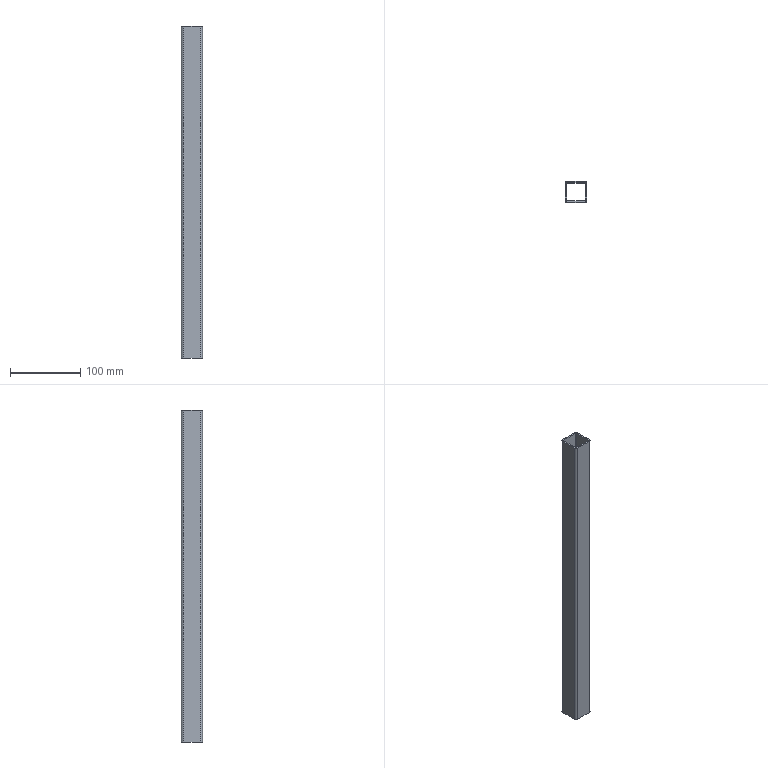Part | STEP file | DIN EN 10305-5 - 30 x 30 x 2  - 473 | 1 solid | 18 faces | box 30 x 30 x 473 mm | volume 102704 mm3 | plane 10 | cylinder 8 | commonest cylinder face diameters 2 x4 6 x4
STEP:
#1=CARTESIAN_POINT('',(0.,0.,0.));
#2=DIRECTION('',(0.,0.,1.));
#3=DIRECTION('',(1.,0.,0.));
#4=AXIS2_PLACEMENT_3D('',#1,#2,#3);
#5=CARTESIAN_POINT('',(-12.,-13.,473.));
#6=VERTEX_POINT('',#5);
#7=CARTESIAN_POINT('',(12.,-13.,473.));
#8=VERTEX_POINT('',#7);
#9=CARTESIAN_POINT('',(6.,-13.,473.));
#10=DIRECTION('',(1.,0.,0.));
#11=VECTOR('',#10,1.);
#12=LINE('',#9,#11);
#13=CARTESIAN_POINT('',(12.,-13.,0.));
#14=DIRECTION('',(0.,-1.,0.));
#15=DIRECTION('',(0.,0.,-1.));
#16=AXIS2_PLACEMENT_3D('',#13,#14,#15);
#17=PLANE('',#16);
#18=CARTESIAN_POINT('',(-473.,-6.));
#19=DIRECTION('',(0.,1.));
#20=VECTOR('',#19,1.);
#21=LINE('',#18,#20);
#22=(GEOMETRIC_REPRESENTATION_CONTEXT(2)PARAMETRIC_REPRESENTATION_CONTEXT()REPRESENTATION_CONTEXT('',''));
#23=DEFINITIONAL_REPRESENTATION('',(#21),#22);
#24=PCURVE('',#17,#23);
#25=CARTESIAN_POINT('',(0.,0.,473.));
#26=DIRECTION('',(0.,0.,1.));
#27=DIRECTION('',(1.,0.,0.));
#28=AXIS2_PLACEMENT_3D('',#25,#26,#27);
#29=PLANE('',#28);
#30=CARTESIAN_POINT('',(6.,-13.));
#31=DIRECTION('',(1.,0.));
#32=VECTOR('',#31,1.);
#33=LINE('',#30,#32);
#34=(GEOMETRIC_REPRESENTATION_CONTEXT(2)PARAMETRIC_REPRESENTATION_CONTEXT()REPRESENTATION_CONTEXT('',''));
#35=DEFINITIONAL_REPRESENTATION('',(#33),#34);
#36=PCURVE('',#29,#35);
#37=SURFACE_CURVE('',#12,(#24,#36),.PCURVE_S1.);
#38=EDGE_CURVE('',#6,#8,#37,.T.);
#39=ORIENTED_EDGE('',*,*,#38,.T.);
#40=CARTESIAN_POINT('',(12.,-13.,0.));
#41=VERTEX_POINT('',#40);
#42=CARTESIAN_POINT('',(12.,-13.,0.));
#43=DIRECTION('',(0.,0.,1.));
#44=VECTOR('',#43,1.);
#45=LINE('',#42,#44);
#46=CARTESIAN_POINT('',(0.,0.));
#47=DIRECTION('',(-1.,0.));
#48=VECTOR('',#47,1.);
#49=LINE('',#46,#48);
#50=(GEOMETRIC_REPRESENTATION_CONTEXT(2)PARAMETRIC_REPRESENTATION_CONTEXT()REPRESENTATION_CONTEXT('',''));
#51=DEFINITIONAL_REPRESENTATION('',(#49),#50);
#52=PCURVE('',#17,#51);
#53=CARTESIAN_POINT('',(12.,-12.,0.));
#54=DIRECTION('',(0.,0.,1.));
#55=DIRECTION('',(0.,1.,0.));
#56=AXIS2_PLACEMENT_3D('',#53,#54,#55);
#57=CYLINDRICAL_SURFACE('',#56,1.);
#58=CARTESIAN_POINT('',(3.142,0.));
#59=DIRECTION('',(0.,1.));
#60=VECTOR('',#59,1.);
#61=LINE('',#58,#60);
#62=(GEOMETRIC_REPRESENTATION_CONTEXT(2)PARAMETRIC_REPRESENTATION_CONTEXT()REPRESENTATION_CONTEXT('',''));
#63=DEFINITIONAL_REPRESENTATION('',(#61),#62);
#64=PCURVE('',#57,#63);
#65=SURFACE_CURVE('',#45,(#52,#64),.PCURVE_S1.);
#66=EDGE_CURVE('',#41,#8,#65,.T.);
#67=ORIENTED_EDGE('',*,*,#66,.F.);
#68=CARTESIAN_POINT('',(-12.,-13.,0.));
#69=VERTEX_POINT('',#68);
#70=CARTESIAN_POINT('',(6.,-13.,0.));
#71=DIRECTION('',(1.,0.,0.));
#72=VECTOR('',#71,1.);
#73=LINE('',#70,#72);
#74=CARTESIAN_POINT('',(0.,-6.));
#75=DIRECTION('',(0.,1.));
#76=VECTOR('',#75,1.);
#77=LINE('',#74,#76);
#78=(GEOMETRIC_REPRESENTATION_CONTEXT(2)PARAMETRIC_REPRESENTATION_CONTEXT()REPRESENTATION_CONTEXT('',''));
#79=DEFINITIONAL_REPRESENTATION('',(#77),#78);
#80=PCURVE('',#17,#79);
#81=CARTESIAN_POINT('',(0.,0.,0.));
#82=DIRECTION('',(0.,0.,1.));
#83=DIRECTION('',(1.,0.,0.));
#84=AXIS2_PLACEMENT_3D('',#81,#82,#83);
#85=PLANE('',#84);
#86=CARTESIAN_POINT('',(6.,-13.));
#87=DIRECTION('',(1.,0.));
#88=VECTOR('',#87,1.);
#89=LINE('',#86,#88);
#90=(GEOMETRIC_REPRESENTATION_CONTEXT(2)PARAMETRIC_REPRESENTATION_CONTEXT()REPRESENTATION_CONTEXT('',''));
#91=DEFINITIONAL_REPRESENTATION('',(#89),#90);
#92=PCURVE('',#85,#91);
#93=SURFACE_CURVE('',#73,(#80,#92),.PCURVE_S1.);
#94=EDGE_CURVE('',#69,#41,#93,.T.);
#95=ORIENTED_EDGE('',*,*,#94,.F.);
#96=CARTESIAN_POINT('',(-12.,-13.,0.));
#97=DIRECTION('',(0.,0.,1.));
#98=VECTOR('',#97,1.);
#99=LINE('',#96,#98);
#100=CARTESIAN_POINT('',(0.,-24.));
#101=DIRECTION('',(-1.,0.));
#102=VECTOR('',#101,1.);
#103=LINE('',#100,#102);
#104=(GEOMETRIC_REPRESENTATION_CONTEXT(2)PARAMETRIC_REPRESENTATION_CONTEXT()REPRESENTATION_CONTEXT('',''));
#105=DEFINITIONAL_REPRESENTATION('',(#103),#104);
#106=PCURVE('',#17,#105);
#107=CARTESIAN_POINT('',(-12.,-12.,0.));
#108=DIRECTION('',(0.,0.,1.));
#109=DIRECTION('',(1.,0.,0.));
#110=AXIS2_PLACEMENT_3D('',#107,#108,#109);
#111=CYLINDRICAL_SURFACE('',#110,1.);
#112=CARTESIAN_POINT('',(4.712,0.));
#113=DIRECTION('',(0.,1.));
#114=VECTOR('',#113,1.);
#115=LINE('',#112,#114);
#116=(GEOMETRIC_REPRESENTATION_CONTEXT(2)PARAMETRIC_REPRESENTATION_CONTEXT()REPRESENTATION_CONTEXT('',''));
#117=DEFINITIONAL_REPRESENTATION('',(#115),#116);
#118=PCURVE('',#111,#117);
#119=SURFACE_CURVE('',#99,(#106,#118),.PCURVE_S1.);
#120=EDGE_CURVE('',#69,#6,#119,.T.);
#121=ORIENTED_EDGE('',*,*,#120,.T.);
#122=EDGE_LOOP('',(#39,#67,#95,#121));
#123=FACE_BOUND('',#122,.T.);
#124=ADVANCED_FACE('',(#123),#17,.F.);
#125=ORIENTED_EDGE('',*,*,#66,.F.);
#126=CARTESIAN_POINT('',(13.,-12.,0.));
#127=VERTEX_POINT('',#126);
#128=CARTESIAN_POINT('',(12.,-12.,0.));
#129=DIRECTION('',(0.,0.,1.));
#130=DIRECTION('',(0.,1.,0.));
#131=AXIS2_PLACEMENT_3D('',#128,#129,#130);
#132=CIRCLE('',#131,1.);
#133=CARTESIAN_POINT('',(0.,0.));
#134=DIRECTION('',(1.,0.));
#135=VECTOR('',#134,1.);
#136=LINE('',#133,#135);
#137=(GEOMETRIC_REPRESENTATION_CONTEXT(2)PARAMETRIC_REPRESENTATION_CONTEXT()REPRESENTATION_CONTEXT('',''));
#138=DEFINITIONAL_REPRESENTATION('',(#136),#137);
#139=PCURVE('',#57,#138);
#140=CARTESIAN_POINT('',(12.,-12.));
#141=DIRECTION('',(0.,1.));
#142=AXIS2_PLACEMENT_2D('',#140,#141);
#143=CIRCLE('',#142,1.);
#144=(GEOMETRIC_REPRESENTATION_CONTEXT(2)PARAMETRIC_REPRESENTATION_CONTEXT()REPRESENTATION_CONTEXT('',''));
#145=DEFINITIONAL_REPRESENTATION('',(#143),#144);
#146=PCURVE('',#85,#145);
#147=SURFACE_CURVE('',#132,(#139,#146),.PCURVE_S1.);
#148=EDGE_CURVE('',#41,#127,#147,.T.);
#149=ORIENTED_EDGE('',*,*,#148,.T.);
#150=CARTESIAN_POINT('',(13.,-12.,473.));
#151=VERTEX_POINT('',#150);
#152=CARTESIAN_POINT('',(13.,-12.,0.));
#153=DIRECTION('',(0.,0.,1.));
#154=VECTOR('',#153,1.);
#155=LINE('',#152,#154);
#156=CARTESIAN_POINT('',(4.712,0.));
#157=DIRECTION('',(0.,1.));
#158=VECTOR('',#157,1.);
#159=LINE('',#156,#158);
#160=(GEOMETRIC_REPRESENTATION_CONTEXT(2)PARAMETRIC_REPRESENTATION_CONTEXT()REPRESENTATION_CONTEXT('',''));
#161=DEFINITIONAL_REPRESENTATION('',(#159),#160);
#162=PCURVE('',#57,#161);
#163=CARTESIAN_POINT('',(13.,12.,0.));
#164=DIRECTION('',(1.,0.,0.));
#165=DIRECTION('',(0.,0.,-1.));
#166=AXIS2_PLACEMENT_3D('',#163,#164,#165);
#167=PLANE('',#166);
#168=CARTESIAN_POINT('',(0.,-24.));
#169=DIRECTION('',(-1.,0.));
#170=VECTOR('',#169,1.);
#171=LINE('',#168,#170);
#172=(GEOMETRIC_REPRESENTATION_CONTEXT(2)PARAMETRIC_REPRESENTATION_CONTEXT()REPRESENTATION_CONTEXT('',''));
#173=DEFINITIONAL_REPRESENTATION('',(#171),#172);
#174=PCURVE('',#167,#173);
#175=SURFACE_CURVE('',#155,(#162,#174),.PCURVE_S1.);
#176=EDGE_CURVE('',#127,#151,#175,.T.);
#177=ORIENTED_EDGE('',*,*,#176,.T.);
#178=CARTESIAN_POINT('',(12.,-12.,473.));
#179=DIRECTION('',(0.,0.,1.));
#180=DIRECTION('',(0.,1.,0.));
#181=AXIS2_PLACEMENT_3D('',#178,#179,#180);
#182=CIRCLE('',#181,1.);
#183=CARTESIAN_POINT('',(0.,473.));
#184=DIRECTION('',(1.,0.));
#185=VECTOR('',#184,1.);
#186=LINE('',#183,#185);
#187=(GEOMETRIC_REPRESENTATION_CONTEXT(2)PARAMETRIC_REPRESENTATION_CONTEXT()REPRESENTATION_CONTEXT('',''));
#188=DEFINITIONAL_REPRESENTATION('',(#186),#187);
#189=PCURVE('',#57,#188);
#190=CARTESIAN_POINT('',(12.,-12.));
#191=DIRECTION('',(0.,1.));
#192=AXIS2_PLACEMENT_2D('',#190,#191);
#193=CIRCLE('',#192,1.);
#194=(GEOMETRIC_REPRESENTATION_CONTEXT(2)PARAMETRIC_REPRESENTATION_CONTEXT()REPRESENTATION_CONTEXT('',''));
#195=DEFINITIONAL_REPRESENTATION('',(#193),#194);
#196=PCURVE('',#29,#195);
#197=SURFACE_CURVE('',#182,(#189,#196),.PCURVE_S1.);
#198=EDGE_CURVE('',#8,#151,#197,.T.);
#199=ORIENTED_EDGE('',*,*,#198,.F.);
#200=EDGE_LOOP('',(#125,#149,#177,#199));
#201=FACE_BOUND('',#200,.F.);
#202=ADVANCED_FACE('',(#201),#57,.F.);
#203=CARTESIAN_POINT('',(13.,12.,473.));
#204=VERTEX_POINT('',#203);
#205=CARTESIAN_POINT('',(13.,6.,473.));
#206=DIRECTION('',(0.,1.,0.));
#207=VECTOR('',#206,1.);
#208=LINE('',#205,#207);
#209=CARTESIAN_POINT('',(-473.,-6.));
#210=DIRECTION('',(0.,1.));
#211=VECTOR('',#210,1.);
#212=LINE('',#209,#211);
#213=(GEOMETRIC_REPRESENTATION_CONTEXT(2)PARAMETRIC_REPRESENTATION_CONTEXT()REPRESENTATION_CONTEXT('',''));
#214=DEFINITIONAL_REPRESENTATION('',(#212),#213);
#215=PCURVE('',#167,#214);
#216=CARTESIAN_POINT('',(13.,6.));
#217=DIRECTION('',(0.,1.));
#218=VECTOR('',#217,1.);
#219=LINE('',#216,#218);
#220=(GEOMETRIC_REPRESENTATION_CONTEXT(2)PARAMETRIC_REPRESENTATION_CONTEXT()REPRESENTATION_CONTEXT('',''));
#221=DEFINITIONAL_REPRESENTATION('',(#219),#220);
#222=PCURVE('',#29,#221);
#223=SURFACE_CURVE('',#208,(#215,#222),.PCURVE_S1.);
#224=EDGE_CURVE('',#151,#204,#223,.T.);
#225=ORIENTED_EDGE('',*,*,#224,.T.);
#226=CARTESIAN_POINT('',(13.,12.,0.));
#227=VERTEX_POINT('',#226);
#228=CARTESIAN_POINT('',(13.,12.,0.));
#229=DIRECTION('',(0.,0.,1.));
#230=VECTOR('',#229,1.);
#231=LINE('',#228,#230);
#232=CARTESIAN_POINT('',(0.,0.));
#233=DIRECTION('',(-1.,0.));
#234=VECTOR('',#233,1.);
#235=LINE('',#232,#234);
#236=(GEOMETRIC_REPRESENTATION_CONTEXT(2)PARAMETRIC_REPRESENTATION_CONTEXT()REPRESENTATION_CONTEXT('',''));
#237=DEFINITIONAL_REPRESENTATION('',(#235),#236);
#238=PCURVE('',#167,#237);
#239=CARTESIAN_POINT('',(12.,12.,0.));
#240=DIRECTION('',(0.,0.,1.));
#241=DIRECTION('',(-1.,0.,0.));
#242=AXIS2_PLACEMENT_3D('',#239,#240,#241);
#243=CYLINDRICAL_SURFACE('',#242,1.);
#244=CARTESIAN_POINT('',(3.142,0.));
#245=DIRECTION('',(0.,1.));
#246=VECTOR('',#245,1.);
#247=LINE('',#244,#246);
#248=(GEOMETRIC_REPRESENTATION_CONTEXT(2)PARAMETRIC_REPRESENTATION_CONTEXT()REPRESENTATION_CONTEXT('',''));
#249=DEFINITIONAL_REPRESENTATION('',(#247),#248);
#250=PCURVE('',#243,#249);
#251=SURFACE_CURVE('',#231,(#238,#250),.PCURVE_S1.);
#252=EDGE_CURVE('',#227,#204,#251,.T.);
#253=ORIENTED_EDGE('',*,*,#252,.F.);
#254=CARTESIAN_POINT('',(13.,6.,0.));
#255=DIRECTION('',(0.,1.,0.));
#256=VECTOR('',#255,1.);
#257=LINE('',#254,#256);
#258=CARTESIAN_POINT('',(0.,-6.));
#259=DIRECTION('',(0.,1.));
#260=VECTOR('',#259,1.);
#261=LINE('',#258,#260);
#262=(GEOMETRIC_REPRESENTATION_CONTEXT(2)PARAMETRIC_REPRESENTATION_CONTEXT()REPRESENTATION_CONTEXT('',''));
#263=DEFINITIONAL_REPRESENTATION('',(#261),#262);
#264=PCURVE('',#167,#263);
#265=CARTESIAN_POINT('',(13.,6.));
#266=DIRECTION('',(0.,1.));
#267=VECTOR('',#266,1.);
#268=LINE('',#265,#267);
#269=(GEOMETRIC_REPRESENTATION_CONTEXT(2)PARAMETRIC_REPRESENTATION_CONTEXT()REPRESENTATION_CONTEXT('',''));
#270=DEFINITIONAL_REPRESENTATION('',(#268),#269);
#271=PCURVE('',#85,#270);
#272=SURFACE_CURVE('',#257,(#264,#271),.PCURVE_S1.);
#273=EDGE_CURVE('',#127,#227,#272,.T.);
#274=ORIENTED_EDGE('',*,*,#273,.F.);
#275=ORIENTED_EDGE('',*,*,#176,.T.);
#276=EDGE_LOOP('',(#225,#253,#274,#275));
#277=FACE_BOUND('',#276,.T.);
#278=ADVANCED_FACE('',(#277),#167,.F.);
#279=ORIENTED_EDGE('',*,*,#252,.F.);
#280=CARTESIAN_POINT('',(12.,13.,0.));
#281=VERTEX_POINT('',#280);
#282=CARTESIAN_POINT('',(12.,12.,0.));
#283=DIRECTION('',(0.,0.,1.));
#284=DIRECTION('',(-1.,0.,0.));
#285=AXIS2_PLACEMENT_3D('',#282,#283,#284);
#286=CIRCLE('',#285,1.);
#287=CARTESIAN_POINT('',(0.,0.));
#288=DIRECTION('',(1.,0.));
#289=VECTOR('',#288,1.);
#290=LINE('',#287,#289);
#291=(GEOMETRIC_REPRESENTATION_CONTEXT(2)PARAMETRIC_REPRESENTATION_CONTEXT()REPRESENTATION_CONTEXT('',''));
#292=DEFINITIONAL_REPRESENTATION('',(#290),#291);
#293=PCURVE('',#243,#292);
#294=CARTESIAN_POINT('',(12.,12.));
#295=DIRECTION('',(-1.,0.));
#296=AXIS2_PLACEMENT_2D('',#294,#295);
#297=CIRCLE('',#296,1.);
#298=(GEOMETRIC_REPRESENTATION_CONTEXT(2)PARAMETRIC_REPRESENTATION_CONTEXT()REPRESENTATION_CONTEXT('',''));
#299=DEFINITIONAL_REPRESENTATION('',(#297),#298);
#300=PCURVE('',#85,#299);
#301=SURFACE_CURVE('',#286,(#293,#300),.PCURVE_S1.);
#302=EDGE_CURVE('',#227,#281,#301,.T.);
#303=ORIENTED_EDGE('',*,*,#302,.T.);
#304=CARTESIAN_POINT('',(12.,13.,473.));
#305=VERTEX_POINT('',#304);
#306=CARTESIAN_POINT('',(12.,13.,0.));
#307=DIRECTION('',(0.,0.,1.));
#308=VECTOR('',#307,1.);
#309=LINE('',#306,#308);
#310=CARTESIAN_POINT('',(4.712,0.));
#311=DIRECTION('',(0.,1.));
#312=VECTOR('',#311,1.);
#313=LINE('',#310,#312);
#314=(GEOMETRIC_REPRESENTATION_CONTEXT(2)PARAMETRIC_REPRESENTATION_CONTEXT()REPRESENTATION_CONTEXT('',''));
#315=DEFINITIONAL_REPRESENTATION('',(#313),#314);
#316=PCURVE('',#243,#315);
#317=CARTESIAN_POINT('',(-12.,13.,0.));
#318=DIRECTION('',(0.,1.,0.));
#319=DIRECTION('',(0.,0.,1.));
#320=AXIS2_PLACEMENT_3D('',#317,#318,#319);
#321=PLANE('',#320);
#322=CARTESIAN_POINT('',(0.,24.));
#323=DIRECTION('',(1.,0.));
#324=VECTOR('',#323,1.);
#325=LINE('',#322,#324);
#326=(GEOMETRIC_REPRESENTATION_CONTEXT(2)PARAMETRIC_REPRESENTATION_CONTEXT()REPRESENTATION_CONTEXT('',''));
#327=DEFINITIONAL_REPRESENTATION('',(#325),#326);
#328=PCURVE('',#321,#327);
#329=SURFACE_CURVE('',#309,(#316,#328),.PCURVE_S1.);
#330=EDGE_CURVE('',#281,#305,#329,.T.);
#331=ORIENTED_EDGE('',*,*,#330,.T.);
#332=CARTESIAN_POINT('',(12.,12.,473.));
#333=DIRECTION('',(0.,0.,1.));
#334=DIRECTION('',(-1.,0.,0.));
#335=AXIS2_PLACEMENT_3D('',#332,#333,#334);
#336=CIRCLE('',#335,1.);
#337=CARTESIAN_POINT('',(0.,473.));
#338=DIRECTION('',(1.,0.));
#339=VECTOR('',#338,1.);
#340=LINE('',#337,#339);
#341=(GEOMETRIC_REPRESENTATION_CONTEXT(2)PARAMETRIC_REPRESENTATION_CONTEXT()REPRESENTATION_CONTEXT('',''));
#342=DEFINITIONAL_REPRESENTATION('',(#340),#341);
#343=PCURVE('',#243,#342);
#344=CARTESIAN_POINT('',(12.,12.));
#345=DIRECTION('',(-1.,0.));
#346=AXIS2_PLACEMENT_2D('',#344,#345);
#347=CIRCLE('',#346,1.);
#348=(GEOMETRIC_REPRESENTATION_CONTEXT(2)PARAMETRIC_REPRESENTATION_CONTEXT()REPRESENTATION_CONTEXT('',''));
#349=DEFINITIONAL_REPRESENTATION('',(#347),#348);
#350=PCURVE('',#29,#349);
#351=SURFACE_CURVE('',#336,(#343,#350),.PCURVE_S1.);
#352=EDGE_CURVE('',#204,#305,#351,.T.);
#353=ORIENTED_EDGE('',*,*,#352,.F.);
#354=EDGE_LOOP('',(#279,#303,#331,#353));
#355=FACE_BOUND('',#354,.F.);
#356=ADVANCED_FACE('',(#355),#243,.F.);
#357=CARTESIAN_POINT('',(15.,12.,473.));
#358=VERTEX_POINT('',#357);
#359=CARTESIAN_POINT('',(15.,-12.,473.));
#360=VERTEX_POINT('',#359);
#361=CARTESIAN_POINT('',(15.,6.,473.));
#362=DIRECTION('',(0.,-1.,0.));
#363=VECTOR('',#362,1.);
#364=LINE('',#361,#363);
#365=CARTESIAN_POINT('',(15.,12.,0.));
#366=DIRECTION('',(1.,0.,0.));
#367=DIRECTION('',(0.,0.,-1.));
#368=AXIS2_PLACEMENT_3D('',#365,#366,#367);
#369=PLANE('',#368);
#370=CARTESIAN_POINT('',(-473.,-6.));
#371=DIRECTION('',(0.,-1.));
#372=VECTOR('',#371,1.);
#373=LINE('',#370,#372);
#374=(GEOMETRIC_REPRESENTATION_CONTEXT(2)PARAMETRIC_REPRESENTATION_CONTEXT()REPRESENTATION_CONTEXT('',''));
#375=DEFINITIONAL_REPRESENTATION('',(#373),#374);
#376=PCURVE('',#369,#375);
#377=CARTESIAN_POINT('',(15.,6.));
#378=DIRECTION('',(0.,-1.));
#379=VECTOR('',#378,1.);
#380=LINE('',#377,#379);
#381=(GEOMETRIC_REPRESENTATION_CONTEXT(2)PARAMETRIC_REPRESENTATION_CONTEXT()REPRESENTATION_CONTEXT('',''));
#382=DEFINITIONAL_REPRESENTATION('',(#380),#381);
#383=PCURVE('',#29,#382);
#384=SURFACE_CURVE('',#364,(#376,#383),.PCURVE_S1.);
#385=EDGE_CURVE('',#358,#360,#384,.T.);
#386=ORIENTED_EDGE('',*,*,#385,.T.);
#387=CARTESIAN_POINT('',(15.,-12.,0.));
#388=VERTEX_POINT('',#387);
#389=CARTESIAN_POINT('',(15.,-12.,0.));
#390=DIRECTION('',(0.,0.,1.));
#391=VECTOR('',#390,1.);
#392=LINE('',#389,#391);
#393=CARTESIAN_POINT('',(0.,-24.));
#394=DIRECTION('',(-1.,0.));
#395=VECTOR('',#394,1.);
#396=LINE('',#393,#395);
#397=(GEOMETRIC_REPRESENTATION_CONTEXT(2)PARAMETRIC_REPRESENTATION_CONTEXT()REPRESENTATION_CONTEXT('',''));
#398=DEFINITIONAL_REPRESENTATION('',(#396),#397);
#399=PCURVE('',#369,#398);
#400=CARTESIAN_POINT('',(12.,-12.,0.));
#401=DIRECTION('',(0.,0.,1.));
#402=DIRECTION('',(0.,1.,0.));
#403=AXIS2_PLACEMENT_3D('',#400,#401,#402);
#404=CYLINDRICAL_SURFACE('',#403,3.);
#405=CARTESIAN_POINT('',(4.712,0.));
#406=DIRECTION('',(0.,1.));
#407=VECTOR('',#406,1.);
#408=LINE('',#405,#407);
#409=(GEOMETRIC_REPRESENTATION_CONTEXT(2)PARAMETRIC_REPRESENTATION_CONTEXT()REPRESENTATION_CONTEXT('',''));
#410=DEFINITIONAL_REPRESENTATION('',(#408),#409);
#411=PCURVE('',#404,#410);
#412=SURFACE_CURVE('',#392,(#399,#411),.PCURVE_S1.);
#413=EDGE_CURVE('',#388,#360,#412,.T.);
#414=ORIENTED_EDGE('',*,*,#413,.F.);
#415=CARTESIAN_POINT('',(15.,12.,0.));
#416=VERTEX_POINT('',#415);
#417=CARTESIAN_POINT('',(15.,6.,0.));
#418=DIRECTION('',(0.,-1.,0.));
#419=VECTOR('',#418,1.);
#420=LINE('',#417,#419);
#421=CARTESIAN_POINT('',(0.,-6.));
#422=DIRECTION('',(0.,-1.));
#423=VECTOR('',#422,1.);
#424=LINE('',#421,#423);
#425=(GEOMETRIC_REPRESENTATION_CONTEXT(2)PARAMETRIC_REPRESENTATION_CONTEXT()REPRESENTATION_CONTEXT('',''));
#426=DEFINITIONAL_REPRESENTATION('',(#424),#425);
#427=PCURVE('',#369,#426);
#428=CARTESIAN_POINT('',(15.,6.));
#429=DIRECTION('',(0.,-1.));
#430=VECTOR('',#429,1.);
#431=LINE('',#428,#430);
#432=(GEOMETRIC_REPRESENTATION_CONTEXT(2)PARAMETRIC_REPRESENTATION_CONTEXT()REPRESENTATION_CONTEXT('',''));
#433=DEFINITIONAL_REPRESENTATION('',(#431),#432);
#434=PCURVE('',#85,#433);
#435=SURFACE_CURVE('',#420,(#427,#434),.PCURVE_S1.);
#436=EDGE_CURVE('',#416,#388,#435,.T.);
#437=ORIENTED_EDGE('',*,*,#436,.F.);
#438=CARTESIAN_POINT('',(15.,12.,0.));
#439=DIRECTION('',(0.,0.,1.));
#440=VECTOR('',#439,1.);
#441=LINE('',#438,#440);
#442=CARTESIAN_POINT('',(0.,0.));
#443=DIRECTION('',(-1.,0.));
#444=VECTOR('',#443,1.);
#445=LINE('',#442,#444);
#446=(GEOMETRIC_REPRESENTATION_CONTEXT(2)PARAMETRIC_REPRESENTATION_CONTEXT()REPRESENTATION_CONTEXT('',''));
#447=DEFINITIONAL_REPRESENTATION('',(#445),#446);
#448=PCURVE('',#369,#447);
#449=CARTESIAN_POINT('',(12.,12.,0.));
#450=DIRECTION('',(0.,0.,1.));
#451=DIRECTION('',(-1.,0.,0.));
#452=AXIS2_PLACEMENT_3D('',#449,#450,#451);
#453=CYLINDRICAL_SURFACE('',#452,3.);
#454=CARTESIAN_POINT('',(3.142,0.));
#455=DIRECTION('',(0.,1.));
#456=VECTOR('',#455,1.);
#457=LINE('',#454,#456);
#458=(GEOMETRIC_REPRESENTATION_CONTEXT(2)PARAMETRIC_REPRESENTATION_CONTEXT()REPRESENTATION_CONTEXT('',''));
#459=DEFINITIONAL_REPRESENTATION('',(#457),#458);
#460=PCURVE('',#453,#459);
#461=SURFACE_CURVE('',#441,(#448,#460),.PCURVE_S1.);
#462=EDGE_CURVE('',#416,#358,#461,.T.);
#463=ORIENTED_EDGE('',*,*,#462,.T.);
#464=EDGE_LOOP('',(#386,#414,#437,#463));
#465=FACE_BOUND('',#464,.T.);
#466=ADVANCED_FACE('',(#465),#369,.T.);
#467=CARTESIAN_POINT('',(12.,-15.,473.));
#468=VERTEX_POINT('',#467);
#469=CARTESIAN_POINT('',(12.,-12.,473.));
#470=DIRECTION('',(0.,0.,-1.));
#471=DIRECTION('',(0.,1.,0.));
#472=AXIS2_PLACEMENT_3D('',#469,#470,#471);
#473=CIRCLE('',#472,3.);
#474=CARTESIAN_POINT('',(6.283,473.));
#475=DIRECTION('',(-1.,0.));
#476=VECTOR('',#475,1.);
#477=LINE('',#474,#476);
#478=(GEOMETRIC_REPRESENTATION_CONTEXT(2)PARAMETRIC_REPRESENTATION_CONTEXT()REPRESENTATION_CONTEXT('',''));
#479=DEFINITIONAL_REPRESENTATION('',(#477),#478);
#480=PCURVE('',#404,#479);
#481=CARTESIAN_POINT('',(12.,-9.));
#482=CARTESIAN_POINT('',(17.196,-9.));
#483=CARTESIAN_POINT('',(14.598,-13.5));
#484=CARTESIAN_POINT('',(12.,-18.));
#485=CARTESIAN_POINT('',(9.402,-13.5));
#486=CARTESIAN_POINT('',(6.804,-9.));
#487=CARTESIAN_POINT('',(12.,-9.));
#488=(BOUNDED_CURVE()B_SPLINE_CURVE(2,(#481,#482,#483,#484,#485,#486,#487),.UNSPECIFIED.,.T.,.F.)B_SPLINE_CURVE_WITH_KNOTS((1,2,2,2,2,1),(-2.094,0.,2.094,4.189,6.283,8.378),.UNSPECIFIED.)CURVE()GEOMETRIC_REPRESENTATION_ITEM()RATIONAL_B_SPLINE_CURVE((1.,0.5,1.,0.5,1.,0.5,1.))REPRESENTATION_ITEM(''));
#489=(GEOMETRIC_REPRESENTATION_CONTEXT(2)PARAMETRIC_REPRESENTATION_CONTEXT()REPRESENTATION_CONTEXT('',''));
#490=DEFINITIONAL_REPRESENTATION('',(#488),#489);
#491=PCURVE('',#29,#490);
#492=SURFACE_CURVE('',#473,(#480,#491),.PCURVE_S1.);
#493=EDGE_CURVE('',#360,#468,#492,.T.);
#494=ORIENTED_EDGE('',*,*,#493,.T.);
#495=CARTESIAN_POINT('',(12.,-15.,0.));
#496=VERTEX_POINT('',#495);
#497=CARTESIAN_POINT('',(12.,-15.,0.));
#498=DIRECTION('',(0.,0.,1.));
#499=VECTOR('',#498,1.);
#500=LINE('',#497,#499);
#501=CARTESIAN_POINT('',(3.142,0.));
#502=DIRECTION('',(0.,1.));
#503=VECTOR('',#502,1.);
#504=LINE('',#501,#503);
#505=(GEOMETRIC_REPRESENTATION_CONTEXT(2)PARAMETRIC_REPRESENTATION_CONTEXT()REPRESENTATION_CONTEXT('',''));
#506=DEFINITIONAL_REPRESENTATION('',(#504),#505);
#507=PCURVE('',#404,#506);
#508=CARTESIAN_POINT('',(12.,-15.,0.));
#509=DIRECTION('',(0.,-1.,0.));
#510=DIRECTION('',(0.,0.,-1.));
#511=AXIS2_PLACEMENT_3D('',#508,#509,#510);
#512=PLANE('',#511);
#513=CARTESIAN_POINT('',(0.,0.));
#514=DIRECTION('',(-1.,0.));
#515=VECTOR('',#514,1.);
#516=LINE('',#513,#515);
#517=(GEOMETRIC_REPRESENTATION_CONTEXT(2)PARAMETRIC_REPRESENTATION_CONTEXT()REPRESENTATION_CONTEXT('',''));
#518=DEFINITIONAL_REPRESENTATION('',(#516),#517);
#519=PCURVE('',#512,#518);
#520=SURFACE_CURVE('',#500,(#507,#519),.PCURVE_S1.);
#521=EDGE_CURVE('',#496,#468,#520,.T.);
#522=ORIENTED_EDGE('',*,*,#521,.F.);
#523=CARTESIAN_POINT('',(12.,-12.,0.));
#524=DIRECTION('',(0.,0.,-1.));
#525=DIRECTION('',(0.,1.,0.));
#526=AXIS2_PLACEMENT_3D('',#523,#524,#525);
#527=CIRCLE('',#526,3.);
#528=CARTESIAN_POINT('',(6.283,0.));
#529=DIRECTION('',(-1.,0.));
#530=VECTOR('',#529,1.);
#531=LINE('',#528,#530);
#532=(GEOMETRIC_REPRESENTATION_CONTEXT(2)PARAMETRIC_REPRESENTATION_CONTEXT()REPRESENTATION_CONTEXT('',''));
#533=DEFINITIONAL_REPRESENTATION('',(#531),#532);
#534=PCURVE('',#404,#533);
#535=CARTESIAN_POINT('',(12.,-9.));
#536=CARTESIAN_POINT('',(17.196,-9.));
#537=CARTESIAN_POINT('',(14.598,-13.5));
#538=CARTESIAN_POINT('',(12.,-18.));
#539=CARTESIAN_POINT('',(9.402,-13.5));
#540=CARTESIAN_POINT('',(6.804,-9.));
#541=CARTESIAN_POINT('',(12.,-9.));
#542=(BOUNDED_CURVE()B_SPLINE_CURVE(2,(#535,#536,#537,#538,#539,#540,#541),.UNSPECIFIED.,.T.,.F.)B_SPLINE_CURVE_WITH_KNOTS((1,2,2,2,2,1),(-2.094,0.,2.094,4.189,6.283,8.378),.UNSPECIFIED.)CURVE()GEOMETRIC_REPRESENTATION_ITEM()RATIONAL_B_SPLINE_CURVE((1.,0.5,1.,0.5,1.,0.5,1.))REPRESENTATION_ITEM(''));
#543=(GEOMETRIC_REPRESENTATION_CONTEXT(2)PARAMETRIC_REPRESENTATION_CONTEXT()REPRESENTATION_CONTEXT('',''));
#544=DEFINITIONAL_REPRESENTATION('',(#542),#543);
#545=PCURVE('',#85,#544);
#546=SURFACE_CURVE('',#527,(#534,#545),.PCURVE_S1.);
#547=EDGE_CURVE('',#388,#496,#546,.T.);
#548=ORIENTED_EDGE('',*,*,#547,.F.);
#549=ORIENTED_EDGE('',*,*,#413,.T.);
#550=EDGE_LOOP('',(#494,#522,#548,#549));
#551=FACE_BOUND('',#550,.T.);
#552=ADVANCED_FACE('',(#551),#404,.T.);
#553=CARTESIAN_POINT('',(-12.,-15.,473.));
#554=VERTEX_POINT('',#553);
#555=CARTESIAN_POINT('',(6.,-15.,473.));
#556=DIRECTION('',(-1.,0.,0.));
#557=VECTOR('',#556,1.);
#558=LINE('',#555,#557);
#559=CARTESIAN_POINT('',(-473.,-6.));
#560=DIRECTION('',(0.,-1.));
#561=VECTOR('',#560,1.);
#562=LINE('',#559,#561);
#563=(GEOMETRIC_REPRESENTATION_CONTEXT(2)PARAMETRIC_REPRESENTATION_CONTEXT()REPRESENTATION_CONTEXT('',''));
#564=DEFINITIONAL_REPRESENTATION('',(#562),#563);
#565=PCURVE('',#512,#564);
#566=CARTESIAN_POINT('',(6.,-15.));
#567=DIRECTION('',(-1.,0.));
#568=VECTOR('',#567,1.);
#569=LINE('',#566,#568);
#570=(GEOMETRIC_REPRESENTATION_CONTEXT(2)PARAMETRIC_REPRESENTATION_CONTEXT()REPRESENTATION_CONTEXT('',''));
#571=DEFINITIONAL_REPRESENTATION('',(#569),#570);
#572=PCURVE('',#29,#571);
#573=SURFACE_CURVE('',#558,(#565,#572),.PCURVE_S1.);
#574=EDGE_CURVE('',#468,#554,#573,.T.);
#575=ORIENTED_EDGE('',*,*,#574,.T.);
#576=CARTESIAN_POINT('',(-12.,-15.,0.));
#577=VERTEX_POINT('',#576);
#578=CARTESIAN_POINT('',(-12.,-15.,0.));
#579=DIRECTION('',(0.,0.,1.));
#580=VECTOR('',#579,1.);
#581=LINE('',#578,#580);
#582=CARTESIAN_POINT('',(0.,-24.));
#583=DIRECTION('',(-1.,0.));
#584=VECTOR('',#583,1.);
#585=LINE('',#582,#584);
#586=(GEOMETRIC_REPRESENTATION_CONTEXT(2)PARAMETRIC_REPRESENTATION_CONTEXT()REPRESENTATION_CONTEXT('',''));
#587=DEFINITIONAL_REPRESENTATION('',(#585),#586);
#588=PCURVE('',#512,#587);
#589=CARTESIAN_POINT('',(-12.,-12.,0.));
#590=DIRECTION('',(0.,0.,1.));
#591=DIRECTION('',(1.,0.,0.));
#592=AXIS2_PLACEMENT_3D('',#589,#590,#591);
#593=CYLINDRICAL_SURFACE('',#592,3.);
#594=CARTESIAN_POINT('',(4.712,0.));
#595=DIRECTION('',(0.,1.));
#596=VECTOR('',#595,1.);
#597=LINE('',#594,#596);
#598=(GEOMETRIC_REPRESENTATION_CONTEXT(2)PARAMETRIC_REPRESENTATION_CONTEXT()REPRESENTATION_CONTEXT('',''));
#599=DEFINITIONAL_REPRESENTATION('',(#597),#598);
#600=PCURVE('',#593,#599);
#601=SURFACE_CURVE('',#581,(#588,#600),.PCURVE_S1.);
#602=EDGE_CURVE('',#577,#554,#601,.T.);
#603=ORIENTED_EDGE('',*,*,#602,.F.);
#604=CARTESIAN_POINT('',(6.,-15.,0.));
#605=DIRECTION('',(-1.,0.,0.));
#606=VECTOR('',#605,1.);
#607=LINE('',#604,#606);
#608=CARTESIAN_POINT('',(0.,-6.));
#609=DIRECTION('',(0.,-1.));
#610=VECTOR('',#609,1.);
#611=LINE('',#608,#610);
#612=(GEOMETRIC_REPRESENTATION_CONTEXT(2)PARAMETRIC_REPRESENTATION_CONTEXT()REPRESENTATION_CONTEXT('',''));
#613=DEFINITIONAL_REPRESENTATION('',(#611),#612);
#614=PCURVE('',#512,#613);
#615=CARTESIAN_POINT('',(6.,-15.));
#616=DIRECTION('',(-1.,0.));
#617=VECTOR('',#616,1.);
#618=LINE('',#615,#617);
#619=(GEOMETRIC_REPRESENTATION_CONTEXT(2)PARAMETRIC_REPRESENTATION_CONTEXT()REPRESENTATION_CONTEXT('',''));
#620=DEFINITIONAL_REPRESENTATION('',(#618),#619);
#621=PCURVE('',#85,#620);
#622=SURFACE_CURVE('',#607,(#614,#621),.PCURVE_S1.);
#623=EDGE_CURVE('',#496,#577,#622,.T.);
#624=ORIENTED_EDGE('',*,*,#623,.F.);
#625=ORIENTED_EDGE('',*,*,#521,.T.);
#626=EDGE_LOOP('',(#575,#603,#624,#625));
#627=FACE_BOUND('',#626,.T.);
#628=ADVANCED_FACE('',(#627),#512,.T.);
#629=CARTESIAN_POINT('',(-15.,-12.,473.));
#630=VERTEX_POINT('',#629);
#631=CARTESIAN_POINT('',(-12.,-12.,473.));
#632=DIRECTION('',(0.,0.,-1.));
#633=DIRECTION('',(1.,0.,0.));
#634=AXIS2_PLACEMENT_3D('',#631,#632,#633);
#635=CIRCLE('',#634,3.);
#636=CARTESIAN_POINT('',(6.283,473.));
#637=DIRECTION('',(-1.,0.));
#638=VECTOR('',#637,1.);
#639=LINE('',#636,#638);
#640=(GEOMETRIC_REPRESENTATION_CONTEXT(2)PARAMETRIC_REPRESENTATION_CONTEXT()REPRESENTATION_CONTEXT('',''));
#641=DEFINITIONAL_REPRESENTATION('',(#639),#640);
#642=PCURVE('',#593,#641);
#643=CARTESIAN_POINT('',(-9.,-12.));
#644=CARTESIAN_POINT('',(-9.,-17.196));
#645=CARTESIAN_POINT('',(-13.5,-14.598));
#646=CARTESIAN_POINT('',(-18.,-12.));
#647=CARTESIAN_POINT('',(-13.5,-9.402));
#648=CARTESIAN_POINT('',(-9.,-6.804));
#649=CARTESIAN_POINT('',(-9.,-12.));
#650=(BOUNDED_CURVE()B_SPLINE_CURVE(2,(#643,#644,#645,#646,#647,#648,#649),.UNSPECIFIED.,.T.,.F.)B_SPLINE_CURVE_WITH_KNOTS((1,2,2,2,2,1),(-2.094,0.,2.094,4.189,6.283,8.378),.UNSPECIFIED.)CURVE()GEOMETRIC_REPRESENTATION_ITEM()RATIONAL_B_SPLINE_CURVE((1.,0.5,1.,0.5,1.,0.5,1.))REPRESENTATION_ITEM(''));
#651=(GEOMETRIC_REPRESENTATION_CONTEXT(2)PARAMETRIC_REPRESENTATION_CONTEXT()REPRESENTATION_CONTEXT('',''));
#652=DEFINITIONAL_REPRESENTATION('',(#650),#651);
#653=PCURVE('',#29,#652);
#654=SURFACE_CURVE('',#635,(#642,#653),.PCURVE_S1.);
#655=EDGE_CURVE('',#554,#630,#654,.T.);
#656=ORIENTED_EDGE('',*,*,#655,.T.);
#657=CARTESIAN_POINT('',(-15.,-12.,0.));
#658=VERTEX_POINT('',#657);
#659=CARTESIAN_POINT('',(-15.,-12.,0.));
#660=DIRECTION('',(0.,0.,1.));
#661=VECTOR('',#660,1.);
#662=LINE('',#659,#661);
#663=CARTESIAN_POINT('',(3.142,0.));
#664=DIRECTION('',(0.,1.));
#665=VECTOR('',#664,1.);
#666=LINE('',#663,#665);
#667=(GEOMETRIC_REPRESENTATION_CONTEXT(2)PARAMETRIC_REPRESENTATION_CONTEXT()REPRESENTATION_CONTEXT('',''));
#668=DEFINITIONAL_REPRESENTATION('',(#666),#667);
#669=PCURVE('',#593,#668);
#670=CARTESIAN_POINT('',(-15.,-12.,0.));
#671=DIRECTION('',(-1.,0.,0.));
#672=DIRECTION('',(0.,0.,1.));
#673=AXIS2_PLACEMENT_3D('',#670,#671,#672);
#674=PLANE('',#673);
#675=CARTESIAN_POINT('',(0.,0.));
#676=DIRECTION('',(1.,0.));
#677=VECTOR('',#676,1.);
#678=LINE('',#675,#677);
#679=(GEOMETRIC_REPRESENTATION_CONTEXT(2)PARAMETRIC_REPRESENTATION_CONTEXT()REPRESENTATION_CONTEXT('',''));
#680=DEFINITIONAL_REPRESENTATION('',(#678),#679);
#681=PCURVE('',#674,#680);
#682=SURFACE_CURVE('',#662,(#669,#681),.PCURVE_S1.);
#683=EDGE_CURVE('',#658,#630,#682,.T.);
#684=ORIENTED_EDGE('',*,*,#683,.F.);
#685=CARTESIAN_POINT('',(-12.,-12.,0.));
#686=DIRECTION('',(0.,0.,-1.));
#687=DIRECTION('',(1.,0.,0.));
#688=AXIS2_PLACEMENT_3D('',#685,#686,#687);
#689=CIRCLE('',#688,3.);
#690=CARTESIAN_POINT('',(6.283,0.));
#691=DIRECTION('',(-1.,0.));
#692=VECTOR('',#691,1.);
#693=LINE('',#690,#692);
#694=(GEOMETRIC_REPRESENTATION_CONTEXT(2)PARAMETRIC_REPRESENTATION_CONTEXT()REPRESENTATION_CONTEXT('',''));
#695=DEFINITIONAL_REPRESENTATION('',(#693),#694);
#696=PCURVE('',#593,#695);
#697=CARTESIAN_POINT('',(-9.,-12.));
#698=CARTESIAN_POINT('',(-9.,-17.196));
#699=CARTESIAN_POINT('',(-13.5,-14.598));
#700=CARTESIAN_POINT('',(-18.,-12.));
#701=CARTESIAN_POINT('',(-13.5,-9.402));
#702=CARTESIAN_POINT('',(-9.,-6.804));
#703=CARTESIAN_POINT('',(-9.,-12.));
#704=(BOUNDED_CURVE()B_SPLINE_CURVE(2,(#697,#698,#699,#700,#701,#702,#703),.UNSPECIFIED.,.T.,.F.)B_SPLINE_CURVE_WITH_KNOTS((1,2,2,2,2,1),(-2.094,0.,2.094,4.189,6.283,8.378),.UNSPECIFIED.)CURVE()GEOMETRIC_REPRESENTATION_ITEM()RATIONAL_B_SPLINE_CURVE((1.,0.5,1.,0.5,1.,0.5,1.))REPRESENTATION_ITEM(''));
#705=(GEOMETRIC_REPRESENTATION_CONTEXT(2)PARAMETRIC_REPRESENTATION_CONTEXT()REPRESENTATION_CONTEXT('',''));
#706=DEFINITIONAL_REPRESENTATION('',(#704),#705);
#707=PCURVE('',#85,#706);
#708=SURFACE_CURVE('',#689,(#696,#707),.PCURVE_S1.);
#709=EDGE_CURVE('',#577,#658,#708,.T.);
#710=ORIENTED_EDGE('',*,*,#709,.F.);
#711=ORIENTED_EDGE('',*,*,#602,.T.);
#712=EDGE_LOOP('',(#656,#684,#710,#711));
#713=FACE_BOUND('',#712,.T.);
#714=ADVANCED_FACE('',(#713),#593,.T.);
#715=CARTESIAN_POINT('',(-12.,13.,473.));
#716=VERTEX_POINT('',#715);
#717=CARTESIAN_POINT('',(-6.,13.,473.));
#718=DIRECTION('',(-1.,0.,0.));
#719=VECTOR('',#718,1.);
#720=LINE('',#717,#719);
#721=CARTESIAN_POINT('',(473.,6.));
#722=DIRECTION('',(0.,-1.));
#723=VECTOR('',#722,1.);
#724=LINE('',#721,#723);
#725=(GEOMETRIC_REPRESENTATION_CONTEXT(2)PARAMETRIC_REPRESENTATION_CONTEXT()REPRESENTATION_CONTEXT('',''));
#726=DEFINITIONAL_REPRESENTATION('',(#724),#725);
#727=PCURVE('',#321,#726);
#728=CARTESIAN_POINT('',(-6.,13.));
#729=DIRECTION('',(-1.,0.));
#730=VECTOR('',#729,1.);
#731=LINE('',#728,#730);
#732=(GEOMETRIC_REPRESENTATION_CONTEXT(2)PARAMETRIC_REPRESENTATION_CONTEXT()REPRESENTATION_CONTEXT('',''));
#733=DEFINITIONAL_REPRESENTATION('',(#731),#732);
#734=PCURVE('',#29,#733);
#735=SURFACE_CURVE('',#720,(#727,#734),.PCURVE_S1.);
#736=EDGE_CURVE('',#305,#716,#735,.T.);
#737=ORIENTED_EDGE('',*,*,#736,.T.);
#738=CARTESIAN_POINT('',(-12.,13.,0.));
#739=VERTEX_POINT('',#738);
#740=CARTESIAN_POINT('',(-12.,13.,0.));
#741=DIRECTION('',(0.,0.,1.));
#742=VECTOR('',#741,1.);
#743=LINE('',#740,#742);
#744=CARTESIAN_POINT('',(0.,0.));
#745=DIRECTION('',(1.,0.));
#746=VECTOR('',#745,1.);
#747=LINE('',#744,#746);
#748=(GEOMETRIC_REPRESENTATION_CONTEXT(2)PARAMETRIC_REPRESENTATION_CONTEXT()REPRESENTATION_CONTEXT('',''));
#749=DEFINITIONAL_REPRESENTATION('',(#747),#748);
#750=PCURVE('',#321,#749);
#751=CARTESIAN_POINT('',(-12.,12.,0.));
#752=DIRECTION('',(0.,0.,1.));
#753=DIRECTION('',(0.,-1.,0.));
#754=AXIS2_PLACEMENT_3D('',#751,#752,#753);
#755=CYLINDRICAL_SURFACE('',#754,1.);
#756=CARTESIAN_POINT('',(3.142,0.));
#757=DIRECTION('',(0.,1.));
#758=VECTOR('',#757,1.);
#759=LINE('',#756,#758);
#760=(GEOMETRIC_REPRESENTATION_CONTEXT(2)PARAMETRIC_REPRESENTATION_CONTEXT()REPRESENTATION_CONTEXT('',''));
#761=DEFINITIONAL_REPRESENTATION('',(#759),#760);
#762=PCURVE('',#755,#761);
#763=SURFACE_CURVE('',#743,(#750,#762),.PCURVE_S1.);
#764=EDGE_CURVE('',#739,#716,#763,.T.);
#765=ORIENTED_EDGE('',*,*,#764,.F.);
#766=CARTESIAN_POINT('',(-6.,13.,0.));
#767=DIRECTION('',(-1.,0.,0.));
#768=VECTOR('',#767,1.);
#769=LINE('',#766,#768);
#770=CARTESIAN_POINT('',(0.,6.));
#771=DIRECTION('',(0.,-1.));
#772=VECTOR('',#771,1.);
#773=LINE('',#770,#772);
#774=(GEOMETRIC_REPRESENTATION_CONTEXT(2)PARAMETRIC_REPRESENTATION_CONTEXT()REPRESENTATION_CONTEXT('',''));
#775=DEFINITIONAL_REPRESENTATION('',(#773),#774);
#776=PCURVE('',#321,#775);
#777=CARTESIAN_POINT('',(-6.,13.));
#778=DIRECTION('',(-1.,0.));
#779=VECTOR('',#778,1.);
#780=LINE('',#777,#779);
#781=(GEOMETRIC_REPRESENTATION_CONTEXT(2)PARAMETRIC_REPRESENTATION_CONTEXT()REPRESENTATION_CONTEXT('',''));
#782=DEFINITIONAL_REPRESENTATION('',(#780),#781);
#783=PCURVE('',#85,#782);
#784=SURFACE_CURVE('',#769,(#776,#783),.PCURVE_S1.);
#785=EDGE_CURVE('',#281,#739,#784,.T.);
#786=ORIENTED_EDGE('',*,*,#785,.F.);
#787=ORIENTED_EDGE('',*,*,#330,.T.);
#788=EDGE_LOOP('',(#737,#765,#786,#787));
#789=FACE_BOUND('',#788,.T.);
#790=ADVANCED_FACE('',(#789),#321,.F.);
#791=CARTESIAN_POINT('',(-13.,-12.,0.));
#792=VERTEX_POINT('',#791);
#793=CARTESIAN_POINT('',(-13.,-12.,473.));
#794=VERTEX_POINT('',#793);
#795=CARTESIAN_POINT('',(-13.,-12.,0.));
#796=DIRECTION('',(0.,0.,1.));
#797=VECTOR('',#796,1.);
#798=LINE('',#795,#797);
#799=CARTESIAN_POINT('',(3.142,0.));
#800=DIRECTION('',(0.,1.));
#801=VECTOR('',#800,1.);
#802=LINE('',#799,#801);
#803=(GEOMETRIC_REPRESENTATION_CONTEXT(2)PARAMETRIC_REPRESENTATION_CONTEXT()REPRESENTATION_CONTEXT('',''));
#804=DEFINITIONAL_REPRESENTATION('',(#802),#803);
#805=PCURVE('',#111,#804);
#806=CARTESIAN_POINT('',(-13.,-12.,0.));
#807=DIRECTION('',(-1.,0.,0.));
#808=DIRECTION('',(0.,0.,1.));
#809=AXIS2_PLACEMENT_3D('',#806,#807,#808);
#810=PLANE('',#809);
#811=CARTESIAN_POINT('',(0.,0.));
#812=DIRECTION('',(1.,0.));
#813=VECTOR('',#812,1.);
#814=LINE('',#811,#813);
#815=(GEOMETRIC_REPRESENTATION_CONTEXT(2)PARAMETRIC_REPRESENTATION_CONTEXT()REPRESENTATION_CONTEXT('',''));
#816=DEFINITIONAL_REPRESENTATION('',(#814),#815);
#817=PCURVE('',#810,#816);
#818=SURFACE_CURVE('',#798,(#805,#817),.PCURVE_S1.);
#819=EDGE_CURVE('',#792,#794,#818,.T.);
#820=ORIENTED_EDGE('',*,*,#819,.F.);
#821=CARTESIAN_POINT('',(-12.,-12.,0.));
#822=DIRECTION('',(0.,0.,1.));
#823=DIRECTION('',(1.,0.,0.));
#824=AXIS2_PLACEMENT_3D('',#821,#822,#823);
#825=CIRCLE('',#824,1.);
#826=CARTESIAN_POINT('',(0.,0.));
#827=DIRECTION('',(1.,0.));
#828=VECTOR('',#827,1.);
#829=LINE('',#826,#828);
#830=(GEOMETRIC_REPRESENTATION_CONTEXT(2)PARAMETRIC_REPRESENTATION_CONTEXT()REPRESENTATION_CONTEXT('',''));
#831=DEFINITIONAL_REPRESENTATION('',(#829),#830);
#832=PCURVE('',#111,#831);
#833=CARTESIAN_POINT('',(-12.,-12.));
#834=DIRECTION('',(1.,0.));
#835=AXIS2_PLACEMENT_2D('',#833,#834);
#836=CIRCLE('',#835,1.);
#837=(GEOMETRIC_REPRESENTATION_CONTEXT(2)PARAMETRIC_REPRESENTATION_CONTEXT()REPRESENTATION_CONTEXT('',''));
#838=DEFINITIONAL_REPRESENTATION('',(#836),#837);
#839=PCURVE('',#85,#838);
#840=SURFACE_CURVE('',#825,(#832,#839),.PCURVE_S1.);
#841=EDGE_CURVE('',#792,#69,#840,.T.);
#842=ORIENTED_EDGE('',*,*,#841,.T.);
#843=ORIENTED_EDGE('',*,*,#120,.T.);
#844=CARTESIAN_POINT('',(-12.,-12.,473.));
#845=DIRECTION('',(0.,0.,1.));
#846=DIRECTION('',(1.,0.,0.));
#847=AXIS2_PLACEMENT_3D('',#844,#845,#846);
#848=CIRCLE('',#847,1.);
#849=CARTESIAN_POINT('',(0.,473.));
#850=DIRECTION('',(1.,0.));
#851=VECTOR('',#850,1.);
#852=LINE('',#849,#851);
#853=(GEOMETRIC_REPRESENTATION_CONTEXT(2)PARAMETRIC_REPRESENTATION_CONTEXT()REPRESENTATION_CONTEXT('',''));
#854=DEFINITIONAL_REPRESENTATION('',(#852),#853);
#855=PCURVE('',#111,#854);
#856=CARTESIAN_POINT('',(-12.,-12.));
#857=DIRECTION('',(1.,0.));
#858=AXIS2_PLACEMENT_2D('',#856,#857);
#859=CIRCLE('',#858,1.);
#860=(GEOMETRIC_REPRESENTATION_CONTEXT(2)PARAMETRIC_REPRESENTATION_CONTEXT()REPRESENTATION_CONTEXT('',''));
#861=DEFINITIONAL_REPRESENTATION('',(#859),#860);
#862=PCURVE('',#29,#861);
#863=SURFACE_CURVE('',#848,(#855,#862),.PCURVE_S1.);
#864=EDGE_CURVE('',#794,#6,#863,.T.);
#865=ORIENTED_EDGE('',*,*,#864,.F.);
#866=EDGE_LOOP('',(#820,#842,#843,#865));
#867=FACE_BOUND('',#866,.F.);
#868=ADVANCED_FACE('',(#867),#111,.F.);
#869=CARTESIAN_POINT('',(-13.,12.,473.));
#870=VERTEX_POINT('',#869);
#871=CARTESIAN_POINT('',(-13.,-6.,473.));
#872=DIRECTION('',(0.,-1.,0.));
#873=VECTOR('',#872,1.);
#874=LINE('',#871,#873);
#875=CARTESIAN_POINT('',(473.,6.));
#876=DIRECTION('',(0.,-1.));
#877=VECTOR('',#876,1.);
#878=LINE('',#875,#877);
#879=(GEOMETRIC_REPRESENTATION_CONTEXT(2)PARAMETRIC_REPRESENTATION_CONTEXT()REPRESENTATION_CONTEXT('',''));
#880=DEFINITIONAL_REPRESENTATION('',(#878),#879);
#881=PCURVE('',#810,#880);
#882=CARTESIAN_POINT('',(-13.,-6.));
#883=DIRECTION('',(0.,-1.));
#884=VECTOR('',#883,1.);
#885=LINE('',#882,#884);
#886=(GEOMETRIC_REPRESENTATION_CONTEXT(2)PARAMETRIC_REPRESENTATION_CONTEXT()REPRESENTATION_CONTEXT('',''));
#887=DEFINITIONAL_REPRESENTATION('',(#885),#886);
#888=PCURVE('',#29,#887);
#889=SURFACE_CURVE('',#874,(#881,#888),.PCURVE_S1.);
#890=EDGE_CURVE('',#870,#794,#889,.T.);
#891=ORIENTED_EDGE('',*,*,#890,.T.);
#892=ORIENTED_EDGE('',*,*,#819,.F.);
#893=CARTESIAN_POINT('',(-13.,12.,0.));
#894=VERTEX_POINT('',#893);
#895=CARTESIAN_POINT('',(-13.,-6.,0.));
#896=DIRECTION('',(0.,-1.,0.));
#897=VECTOR('',#896,1.);
#898=LINE('',#895,#897);
#899=CARTESIAN_POINT('',(0.,6.));
#900=DIRECTION('',(0.,-1.));
#901=VECTOR('',#900,1.);
#902=LINE('',#899,#901);
#903=(GEOMETRIC_REPRESENTATION_CONTEXT(2)PARAMETRIC_REPRESENTATION_CONTEXT()REPRESENTATION_CONTEXT('',''));
#904=DEFINITIONAL_REPRESENTATION('',(#902),#903);
#905=PCURVE('',#810,#904);
#906=CARTESIAN_POINT('',(-13.,-6.));
#907=DIRECTION('',(0.,-1.));
#908=VECTOR('',#907,1.);
#909=LINE('',#906,#908);
#910=(GEOMETRIC_REPRESENTATION_CONTEXT(2)PARAMETRIC_REPRESENTATION_CONTEXT()REPRESENTATION_CONTEXT('',''));
#911=DEFINITIONAL_REPRESENTATION('',(#909),#910);
#912=PCURVE('',#85,#911);
#913=SURFACE_CURVE('',#898,(#905,#912),.PCURVE_S1.);
#914=EDGE_CURVE('',#894,#792,#913,.T.);
#915=ORIENTED_EDGE('',*,*,#914,.F.);
#916=CARTESIAN_POINT('',(-13.,12.,0.));
#917=DIRECTION('',(0.,0.,1.));
#918=VECTOR('',#917,1.);
#919=LINE('',#916,#918);
#920=CARTESIAN_POINT('',(0.,24.));
#921=DIRECTION('',(1.,0.));
#922=VECTOR('',#921,1.);
#923=LINE('',#920,#922);
#924=(GEOMETRIC_REPRESENTATION_CONTEXT(2)PARAMETRIC_REPRESENTATION_CONTEXT()REPRESENTATION_CONTEXT('',''));
#925=DEFINITIONAL_REPRESENTATION('',(#923),#924);
#926=PCURVE('',#810,#925);
#927=CARTESIAN_POINT('',(4.712,0.));
#928=DIRECTION('',(0.,1.));
#929=VECTOR('',#928,1.);
#930=LINE('',#927,#929);
#931=(GEOMETRIC_REPRESENTATION_CONTEXT(2)PARAMETRIC_REPRESENTATION_CONTEXT()REPRESENTATION_CONTEXT('',''));
#932=DEFINITIONAL_REPRESENTATION('',(#930),#931);
#933=PCURVE('',#755,#932);
#934=SURFACE_CURVE('',#919,(#926,#933),.PCURVE_S1.);
#935=EDGE_CURVE('',#894,#870,#934,.T.);
#936=ORIENTED_EDGE('',*,*,#935,.T.);
#937=EDGE_LOOP('',(#891,#892,#915,#936));
#938=FACE_BOUND('',#937,.T.);
#939=ADVANCED_FACE('',(#938),#810,.F.);
#940=ORIENTED_EDGE('',*,*,#764,.F.);
#941=CARTESIAN_POINT('',(-12.,12.,0.));
#942=DIRECTION('',(0.,0.,1.));
#943=DIRECTION('',(0.,-1.,0.));
#944=AXIS2_PLACEMENT_3D('',#941,#942,#943);
#945=CIRCLE('',#944,1.);
#946=CARTESIAN_POINT('',(0.,0.));
#947=DIRECTION('',(1.,0.));
#948=VECTOR('',#947,1.);
#949=LINE('',#946,#948);
#950=(GEOMETRIC_REPRESENTATION_CONTEXT(2)PARAMETRIC_REPRESENTATION_CONTEXT()REPRESENTATION_CONTEXT('',''));
#951=DEFINITIONAL_REPRESENTATION('',(#949),#950);
#952=PCURVE('',#755,#951);
#953=CARTESIAN_POINT('',(-12.,12.));
#954=DIRECTION('',(0.,-1.));
#955=AXIS2_PLACEMENT_2D('',#953,#954);
#956=CIRCLE('',#955,1.);
#957=(GEOMETRIC_REPRESENTATION_CONTEXT(2)PARAMETRIC_REPRESENTATION_CONTEXT()REPRESENTATION_CONTEXT('',''));
#958=DEFINITIONAL_REPRESENTATION('',(#956),#957);
#959=PCURVE('',#85,#958);
#960=SURFACE_CURVE('',#945,(#952,#959),.PCURVE_S1.);
#961=EDGE_CURVE('',#739,#894,#960,.T.);
#962=ORIENTED_EDGE('',*,*,#961,.T.);
#963=ORIENTED_EDGE('',*,*,#935,.T.);
#964=CARTESIAN_POINT('',(-12.,12.,473.));
#965=DIRECTION('',(0.,0.,1.));
#966=DIRECTION('',(0.,-1.,0.));
#967=AXIS2_PLACEMENT_3D('',#964,#965,#966);
#968=CIRCLE('',#967,1.);
#969=CARTESIAN_POINT('',(0.,473.));
#970=DIRECTION('',(1.,0.));
#971=VECTOR('',#970,1.);
#972=LINE('',#969,#971);
#973=(GEOMETRIC_REPRESENTATION_CONTEXT(2)PARAMETRIC_REPRESENTATION_CONTEXT()REPRESENTATION_CONTEXT('',''));
#974=DEFINITIONAL_REPRESENTATION('',(#972),#973);
#975=PCURVE('',#755,#974);
#976=CARTESIAN_POINT('',(-12.,12.));
#977=DIRECTION('',(0.,-1.));
#978=AXIS2_PLACEMENT_2D('',#976,#977);
#979=CIRCLE('',#978,1.);
#980=(GEOMETRIC_REPRESENTATION_CONTEXT(2)PARAMETRIC_REPRESENTATION_CONTEXT()REPRESENTATION_CONTEXT('',''));
#981=DEFINITIONAL_REPRESENTATION('',(#979),#980);
#982=PCURVE('',#29,#981);
#983=SURFACE_CURVE('',#968,(#975,#982),.PCURVE_S1.);
#984=EDGE_CURVE('',#716,#870,#983,.T.);
#985=ORIENTED_EDGE('',*,*,#984,.F.);
#986=EDGE_LOOP('',(#940,#962,#963,#985));
#987=FACE_BOUND('',#986,.F.);
#988=ADVANCED_FACE('',(#987),#755,.F.);
#989=CARTESIAN_POINT('',(-15.,12.,473.));
#990=VERTEX_POINT('',#989);
#991=CARTESIAN_POINT('',(-15.,-6.,473.));
#992=DIRECTION('',(0.,1.,0.));
#993=VECTOR('',#992,1.);
#994=LINE('',#991,#993);
#995=CARTESIAN_POINT('',(473.,6.));
#996=DIRECTION('',(0.,1.));
#997=VECTOR('',#996,1.);
#998=LINE('',#995,#997);
#999=(GEOMETRIC_REPRESENTATION_CONTEXT(2)PARAMETRIC_REPRESENTATION_CONTEXT()REPRESENTATION_CONTEXT('',''));
#1000=DEFINITIONAL_REPRESENTATION('',(#998),#999);
#1001=PCURVE('',#674,#1000);
#1002=CARTESIAN_POINT('',(-15.,-6.));
#1003=DIRECTION('',(0.,1.));
#1004=VECTOR('',#1003,1.);
#1005=LINE('',#1002,#1004);
#1006=(GEOMETRIC_REPRESENTATION_CONTEXT(2)PARAMETRIC_REPRESENTATION_CONTEXT()REPRESENTATION_CONTEXT('',''));
#1007=DEFINITIONAL_REPRESENTATION('',(#1005),#1006);
#1008=PCURVE('',#29,#1007);
#1009=SURFACE_CURVE('',#994,(#1001,#1008),.PCURVE_S1.);
#1010=EDGE_CURVE('',#630,#990,#1009,.T.);
#1011=ORIENTED_EDGE('',*,*,#1010,.T.);
#1012=CARTESIAN_POINT('',(-15.,12.,0.));
#1013=VERTEX_POINT('',#1012);
#1014=CARTESIAN_POINT('',(-15.,12.,0.));
#1015=DIRECTION('',(0.,0.,1.));
#1016=VECTOR('',#1015,1.);
#1017=LINE('',#1014,#1016);
#1018=CARTESIAN_POINT('',(0.,24.));
#1019=DIRECTION('',(1.,0.));
#1020=VECTOR('',#1019,1.);
#1021=LINE('',#1018,#1020);
#1022=(GEOMETRIC_REPRESENTATION_CONTEXT(2)PARAMETRIC_REPRESENTATION_CONTEXT()REPRESENTATION_CONTEXT('',''));
#1023=DEFINITIONAL_REPRESENTATION('',(#1021),#1022);
#1024=PCURVE('',#674,#1023);
#1025=CARTESIAN_POINT('',(-12.,12.,0.));
#1026=DIRECTION('',(0.,0.,1.));
#1027=DIRECTION('',(0.,-1.,0.));
#1028=AXIS2_PLACEMENT_3D('',#1025,#1026,#1027);
#1029=CYLINDRICAL_SURFACE('',#1028,3.);
#1030=CARTESIAN_POINT('',(4.712,0.));
#1031=DIRECTION('',(0.,1.));
#1032=VECTOR('',#1031,1.);
#1033=LINE('',#1030,#1032);
#1034=(GEOMETRIC_REPRESENTATION_CONTEXT(2)PARAMETRIC_REPRESENTATION_CONTEXT()REPRESENTATION_CONTEXT('',''));
#1035=DEFINITIONAL_REPRESENTATION('',(#1033),#1034);
#1036=PCURVE('',#1029,#1035);
#1037=SURFACE_CURVE('',#1017,(#1024,#1036),.PCURVE_S1.);
#1038=EDGE_CURVE('',#1013,#990,#1037,.T.);
#1039=ORIENTED_EDGE('',*,*,#1038,.F.);
#1040=CARTESIAN_POINT('',(-15.,-6.,0.));
#1041=DIRECTION('',(0.,1.,0.));
#1042=VECTOR('',#1041,1.);
#1043=LINE('',#1040,#1042);
#1044=CARTESIAN_POINT('',(0.,6.));
#1045=DIRECTION('',(0.,1.));
#1046=VECTOR('',#1045,1.);
#1047=LINE('',#1044,#1046);
#1048=(GEOMETRIC_REPRESENTATION_CONTEXT(2)PARAMETRIC_REPRESENTATION_CONTEXT()REPRESENTATION_CONTEXT('',''));
#1049=DEFINITIONAL_REPRESENTATION('',(#1047),#1048);
#1050=PCURVE('',#674,#1049);
#1051=CARTESIAN_POINT('',(-15.,-6.));
#1052=DIRECTION('',(0.,1.));
#1053=VECTOR('',#1052,1.);
#1054=LINE('',#1051,#1053);
#1055=(GEOMETRIC_REPRESENTATION_CONTEXT(2)PARAMETRIC_REPRESENTATION_CONTEXT()REPRESENTATION_CONTEXT('',''));
#1056=DEFINITIONAL_REPRESENTATION('',(#1054),#1055);
#1057=PCURVE('',#85,#1056);
#1058=SURFACE_CURVE('',#1043,(#1050,#1057),.PCURVE_S1.);
#1059=EDGE_CURVE('',#658,#1013,#1058,.T.);
#1060=ORIENTED_EDGE('',*,*,#1059,.F.);
#1061=ORIENTED_EDGE('',*,*,#683,.T.);
#1062=EDGE_LOOP('',(#1011,#1039,#1060,#1061));
#1063=FACE_BOUND('',#1062,.T.);
#1064=ADVANCED_FACE('',(#1063),#674,.T.);
#1065=CARTESIAN_POINT('',(-12.,15.,473.));
#1066=VERTEX_POINT('',#1065);
#1067=CARTESIAN_POINT('',(-12.,12.,473.));
#1068=DIRECTION('',(0.,0.,-1.));
#1069=DIRECTION('',(0.,-1.,0.));
#1070=AXIS2_PLACEMENT_3D('',#1067,#1068,#1069);
#1071=CIRCLE('',#1070,3.);
#1072=CARTESIAN_POINT('',(6.283,473.));
#1073=DIRECTION('',(-1.,0.));
#1074=VECTOR('',#1073,1.);
#1075=LINE('',#1072,#1074);
#1076=(GEOMETRIC_REPRESENTATION_CONTEXT(2)PARAMETRIC_REPRESENTATION_CONTEXT()REPRESENTATION_CONTEXT('',''));
#1077=DEFINITIONAL_REPRESENTATION('',(#1075),#1076);
#1078=PCURVE('',#1029,#1077);
#1079=CARTESIAN_POINT('',(-12.,9.));
#1080=CARTESIAN_POINT('',(-17.196,9.));
#1081=CARTESIAN_POINT('',(-14.598,13.5));
#1082=CARTESIAN_POINT('',(-12.,18.));
#1083=CARTESIAN_POINT('',(-9.402,13.5));
#1084=CARTESIAN_POINT('',(-6.804,9.));
#1085=CARTESIAN_POINT('',(-12.,9.));
#1086=(BOUNDED_CURVE()B_SPLINE_CURVE(2,(#1079,#1080,#1081,#1082,#1083,#1084,#1085),.UNSPECIFIED.,.T.,.F.)B_SPLINE_CURVE_WITH_KNOTS((1,2,2,2,2,1),(-2.094,0.,2.094,4.189,6.283,8.378),.UNSPECIFIED.)CURVE()GEOMETRIC_REPRESENTATION_ITEM()RATIONAL_B_SPLINE_CURVE((1.,0.5,1.,0.5,1.,0.5,1.))REPRESENTATION_ITEM(''));
#1087=(GEOMETRIC_REPRESENTATION_CONTEXT(2)PARAMETRIC_REPRESENTATION_CONTEXT()REPRESENTATION_CONTEXT('',''));
#1088=DEFINITIONAL_REPRESENTATION('',(#1086),#1087);
#1089=PCURVE('',#29,#1088);
#1090=SURFACE_CURVE('',#1071,(#1078,#1089),.PCURVE_S1.);
#1091=EDGE_CURVE('',#990,#1066,#1090,.T.);
#1092=ORIENTED_EDGE('',*,*,#1091,.T.);
#1093=CARTESIAN_POINT('',(-12.,15.,0.));
#1094=VERTEX_POINT('',#1093);
#1095=CARTESIAN_POINT('',(-12.,15.,0.));
#1096=DIRECTION('',(0.,0.,1.));
#1097=VECTOR('',#1096,1.);
#1098=LINE('',#1095,#1097);
#1099=CARTESIAN_POINT('',(3.142,0.));
#1100=DIRECTION('',(0.,1.));
#1101=VECTOR('',#1100,1.);
#1102=LINE('',#1099,#1101);
#1103=(GEOMETRIC_REPRESENTATION_CONTEXT(2)PARAMETRIC_REPRESENTATION_CONTEXT()REPRESENTATION_CONTEXT('',''));
#1104=DEFINITIONAL_REPRESENTATION('',(#1102),#1103);
#1105=PCURVE('',#1029,#1104);
#1106=CARTESIAN_POINT('',(-12.,15.,0.));
#1107=DIRECTION('',(0.,1.,0.));
#1108=DIRECTION('',(0.,0.,1.));
#1109=AXIS2_PLACEMENT_3D('',#1106,#1107,#1108);
#1110=PLANE('',#1109);
#1111=CARTESIAN_POINT('',(0.,0.));
#1112=DIRECTION('',(1.,0.));
#1113=VECTOR('',#1112,1.);
#1114=LINE('',#1111,#1113);
#1115=(GEOMETRIC_REPRESENTATION_CONTEXT(2)PARAMETRIC_REPRESENTATION_CONTEXT()REPRESENTATION_CONTEXT('',''));
#1116=DEFINITIONAL_REPRESENTATION('',(#1114),#1115);
#1117=PCURVE('',#1110,#1116);
#1118=SURFACE_CURVE('',#1098,(#1105,#1117),.PCURVE_S1.);
#1119=EDGE_CURVE('',#1094,#1066,#1118,.T.);
#1120=ORIENTED_EDGE('',*,*,#1119,.F.);
#1121=CARTESIAN_POINT('',(-12.,12.,0.));
#1122=DIRECTION('',(0.,0.,-1.));
#1123=DIRECTION('',(0.,-1.,0.));
#1124=AXIS2_PLACEMENT_3D('',#1121,#1122,#1123);
#1125=CIRCLE('',#1124,3.);
#1126=CARTESIAN_POINT('',(6.283,0.));
#1127=DIRECTION('',(-1.,0.));
#1128=VECTOR('',#1127,1.);
#1129=LINE('',#1126,#1128);
#1130=(GEOMETRIC_REPRESENTATION_CONTEXT(2)PARAMETRIC_REPRESENTATION_CONTEXT()REPRESENTATION_CONTEXT('',''));
#1131=DEFINITIONAL_REPRESENTATION('',(#1129),#1130);
#1132=PCURVE('',#1029,#1131);
#1133=CARTESIAN_POINT('',(-12.,9.));
#1134=CARTESIAN_POINT('',(-17.196,9.));
#1135=CARTESIAN_POINT('',(-14.598,13.5));
#1136=CARTESIAN_POINT('',(-12.,18.));
#1137=CARTESIAN_POINT('',(-9.402,13.5));
#1138=CARTESIAN_POINT('',(-6.804,9.));
#1139=CARTESIAN_POINT('',(-12.,9.));
#1140=(BOUNDED_CURVE()B_SPLINE_CURVE(2,(#1133,#1134,#1135,#1136,#1137,#1138,#1139),.UNSPECIFIED.,.T.,.F.)B_SPLINE_CURVE_WITH_KNOTS((1,2,2,2,2,1),(-2.094,0.,2.094,4.189,6.283,8.378),.UNSPECIFIED.)CURVE()GEOMETRIC_REPRESENTATION_ITEM()RATIONAL_B_SPLINE_CURVE((1.,0.5,1.,0.5,1.,0.5,1.))REPRESENTATION_ITEM(''));
#1141=(GEOMETRIC_REPRESENTATION_CONTEXT(2)PARAMETRIC_REPRESENTATION_CONTEXT()REPRESENTATION_CONTEXT('',''));
#1142=DEFINITIONAL_REPRESENTATION('',(#1140),#1141);
#1143=PCURVE('',#85,#1142);
#1144=SURFACE_CURVE('',#1125,(#1132,#1143),.PCURVE_S1.);
#1145=EDGE_CURVE('',#1013,#1094,#1144,.T.);
#1146=ORIENTED_EDGE('',*,*,#1145,.F.);
#1147=ORIENTED_EDGE('',*,*,#1038,.T.);
#1148=EDGE_LOOP('',(#1092,#1120,#1146,#1147));
#1149=FACE_BOUND('',#1148,.T.);
#1150=ADVANCED_FACE('',(#1149),#1029,.T.);
#1151=CARTESIAN_POINT('',(12.,15.,473.));
#1152=VERTEX_POINT('',#1151);
#1153=CARTESIAN_POINT('',(-6.,15.,473.));
#1154=DIRECTION('',(1.,0.,0.));
#1155=VECTOR('',#1154,1.);
#1156=LINE('',#1153,#1155);
#1157=CARTESIAN_POINT('',(473.,6.));
#1158=DIRECTION('',(0.,1.));
#1159=VECTOR('',#1158,1.);
#1160=LINE('',#1157,#1159);
#1161=(GEOMETRIC_REPRESENTATION_CONTEXT(2)PARAMETRIC_REPRESENTATION_CONTEXT()REPRESENTATION_CONTEXT('',''));
#1162=DEFINITIONAL_REPRESENTATION('',(#1160),#1161);
#1163=PCURVE('',#1110,#1162);
#1164=CARTESIAN_POINT('',(-6.,15.));
#1165=DIRECTION('',(1.,0.));
#1166=VECTOR('',#1165,1.);
#1167=LINE('',#1164,#1166);
#1168=(GEOMETRIC_REPRESENTATION_CONTEXT(2)PARAMETRIC_REPRESENTATION_CONTEXT()REPRESENTATION_CONTEXT('',''));
#1169=DEFINITIONAL_REPRESENTATION('',(#1167),#1168);
#1170=PCURVE('',#29,#1169);
#1171=SURFACE_CURVE('',#1156,(#1163,#1170),.PCURVE_S1.);
#1172=EDGE_CURVE('',#1066,#1152,#1171,.T.);
#1173=ORIENTED_EDGE('',*,*,#1172,.T.);
#1174=CARTESIAN_POINT('',(12.,15.,0.));
#1175=VERTEX_POINT('',#1174);
#1176=CARTESIAN_POINT('',(12.,15.,0.));
#1177=DIRECTION('',(0.,0.,1.));
#1178=VECTOR('',#1177,1.);
#1179=LINE('',#1176,#1178);
#1180=CARTESIAN_POINT('',(0.,24.));
#1181=DIRECTION('',(1.,0.));
#1182=VECTOR('',#1181,1.);
#1183=LINE('',#1180,#1182);
#1184=(GEOMETRIC_REPRESENTATION_CONTEXT(2)PARAMETRIC_REPRESENTATION_CONTEXT()REPRESENTATION_CONTEXT('',''));
#1185=DEFINITIONAL_REPRESENTATION('',(#1183),#1184);
#1186=PCURVE('',#1110,#1185);
#1187=CARTESIAN_POINT('',(4.712,0.));
#1188=DIRECTION('',(0.,1.));
#1189=VECTOR('',#1188,1.);
#1190=LINE('',#1187,#1189);
#1191=(GEOMETRIC_REPRESENTATION_CONTEXT(2)PARAMETRIC_REPRESENTATION_CONTEXT()REPRESENTATION_CONTEXT('',''));
#1192=DEFINITIONAL_REPRESENTATION('',(#1190),#1191);
#1193=PCURVE('',#453,#1192);
#1194=SURFACE_CURVE('',#1179,(#1186,#1193),.PCURVE_S1.);
#1195=EDGE_CURVE('',#1175,#1152,#1194,.T.);
#1196=ORIENTED_EDGE('',*,*,#1195,.F.);
#1197=CARTESIAN_POINT('',(-6.,15.,0.));
#1198=DIRECTION('',(1.,0.,0.));
#1199=VECTOR('',#1198,1.);
#1200=LINE('',#1197,#1199);
#1201=CARTESIAN_POINT('',(0.,6.));
#1202=DIRECTION('',(0.,1.));
#1203=VECTOR('',#1202,1.);
#1204=LINE('',#1201,#1203);
#1205=(GEOMETRIC_REPRESENTATION_CONTEXT(2)PARAMETRIC_REPRESENTATION_CONTEXT()REPRESENTATION_CONTEXT('',''));
#1206=DEFINITIONAL_REPRESENTATION('',(#1204),#1205);
#1207=PCURVE('',#1110,#1206);
#1208=CARTESIAN_POINT('',(-6.,15.));
#1209=DIRECTION('',(1.,0.));
#1210=VECTOR('',#1209,1.);
#1211=LINE('',#1208,#1210);
#1212=(GEOMETRIC_REPRESENTATION_CONTEXT(2)PARAMETRIC_REPRESENTATION_CONTEXT()REPRESENTATION_CONTEXT('',''));
#1213=DEFINITIONAL_REPRESENTATION('',(#1211),#1212);
#1214=PCURVE('',#85,#1213);
#1215=SURFACE_CURVE('',#1200,(#1207,#1214),.PCURVE_S1.);
#1216=EDGE_CURVE('',#1094,#1175,#1215,.T.);
#1217=ORIENTED_EDGE('',*,*,#1216,.F.);
#1218=ORIENTED_EDGE('',*,*,#1119,.T.);
#1219=EDGE_LOOP('',(#1173,#1196,#1217,#1218));
#1220=FACE_BOUND('',#1219,.T.);
#1221=ADVANCED_FACE('',(#1220),#1110,.T.);
#1222=CARTESIAN_POINT('',(12.,12.,473.));
#1223=DIRECTION('',(0.,0.,-1.));
#1224=DIRECTION('',(-1.,0.,0.));
#1225=AXIS2_PLACEMENT_3D('',#1222,#1223,#1224);
#1226=CIRCLE('',#1225,3.);
#1227=CARTESIAN_POINT('',(6.283,473.));
#1228=DIRECTION('',(-1.,0.));
#1229=VECTOR('',#1228,1.);
#1230=LINE('',#1227,#1229);
#1231=(GEOMETRIC_REPRESENTATION_CONTEXT(2)PARAMETRIC_REPRESENTATION_CONTEXT()REPRESENTATION_CONTEXT('',''));
#1232=DEFINITIONAL_REPRESENTATION('',(#1230),#1231);
#1233=PCURVE('',#453,#1232);
#1234=CARTESIAN_POINT('',(9.,12.));
#1235=CARTESIAN_POINT('',(9.,17.196));
#1236=CARTESIAN_POINT('',(13.5,14.598));
#1237=CARTESIAN_POINT('',(18.,12.));
#1238=CARTESIAN_POINT('',(13.5,9.402));
#1239=CARTESIAN_POINT('',(9.,6.804));
#1240=CARTESIAN_POINT('',(9.,12.));
#1241=(BOUNDED_CURVE()B_SPLINE_CURVE(2,(#1234,#1235,#1236,#1237,#1238,#1239,#1240),.UNSPECIFIED.,.T.,.F.)B_SPLINE_CURVE_WITH_KNOTS((1,2,2,2,2,1),(-2.094,0.,2.094,4.189,6.283,8.378),.UNSPECIFIED.)CURVE()GEOMETRIC_REPRESENTATION_ITEM()RATIONAL_B_SPLINE_CURVE((1.,0.5,1.,0.5,1.,0.5,1.))REPRESENTATION_ITEM(''));
#1242=(GEOMETRIC_REPRESENTATION_CONTEXT(2)PARAMETRIC_REPRESENTATION_CONTEXT()REPRESENTATION_CONTEXT('',''));
#1243=DEFINITIONAL_REPRESENTATION('',(#1241),#1242);
#1244=PCURVE('',#29,#1243);
#1245=SURFACE_CURVE('',#1226,(#1233,#1244),.PCURVE_S1.);
#1246=EDGE_CURVE('',#1152,#358,#1245,.T.);
#1247=ORIENTED_EDGE('',*,*,#1246,.T.);
#1248=ORIENTED_EDGE('',*,*,#462,.F.);
#1249=CARTESIAN_POINT('',(12.,12.,0.));
#1250=DIRECTION('',(0.,0.,-1.));
#1251=DIRECTION('',(-1.,0.,0.));
#1252=AXIS2_PLACEMENT_3D('',#1249,#1250,#1251);
#1253=CIRCLE('',#1252,3.);
#1254=CARTESIAN_POINT('',(6.283,0.));
#1255=DIRECTION('',(-1.,0.));
#1256=VECTOR('',#1255,1.);
#1257=LINE('',#1254,#1256);
#1258=(GEOMETRIC_REPRESENTATION_CONTEXT(2)PARAMETRIC_REPRESENTATION_CONTEXT()REPRESENTATION_CONTEXT('',''));
#1259=DEFINITIONAL_REPRESENTATION('',(#1257),#1258);
#1260=PCURVE('',#453,#1259);
#1261=CARTESIAN_POINT('',(9.,12.));
#1262=CARTESIAN_POINT('',(9.,17.196));
#1263=CARTESIAN_POINT('',(13.5,14.598));
#1264=CARTESIAN_POINT('',(18.,12.));
#1265=CARTESIAN_POINT('',(13.5,9.402));
#1266=CARTESIAN_POINT('',(9.,6.804));
#1267=CARTESIAN_POINT('',(9.,12.));
#1268=(BOUNDED_CURVE()B_SPLINE_CURVE(2,(#1261,#1262,#1263,#1264,#1265,#1266,#1267),.UNSPECIFIED.,.T.,.F.)B_SPLINE_CURVE_WITH_KNOTS((1,2,2,2,2,1),(-2.094,0.,2.094,4.189,6.283,8.378),.UNSPECIFIED.)CURVE()GEOMETRIC_REPRESENTATION_ITEM()RATIONAL_B_SPLINE_CURVE((1.,0.5,1.,0.5,1.,0.5,1.))REPRESENTATION_ITEM(''));
#1269=(GEOMETRIC_REPRESENTATION_CONTEXT(2)PARAMETRIC_REPRESENTATION_CONTEXT()REPRESENTATION_CONTEXT('',''));
#1270=DEFINITIONAL_REPRESENTATION('',(#1268),#1269);
#1271=PCURVE('',#85,#1270);
#1272=SURFACE_CURVE('',#1253,(#1260,#1271),.PCURVE_S1.);
#1273=EDGE_CURVE('',#1175,#416,#1272,.T.);
#1274=ORIENTED_EDGE('',*,*,#1273,.F.);
#1275=ORIENTED_EDGE('',*,*,#1195,.T.);
#1276=EDGE_LOOP('',(#1247,#1248,#1274,#1275));
#1277=FACE_BOUND('',#1276,.T.);
#1278=ADVANCED_FACE('',(#1277),#453,.T.);
#1279=ORIENTED_EDGE('',*,*,#1059,.T.);
#1280=ORIENTED_EDGE('',*,*,#1145,.T.);
#1281=ORIENTED_EDGE('',*,*,#1216,.T.);
#1282=ORIENTED_EDGE('',*,*,#1273,.T.);
#1283=ORIENTED_EDGE('',*,*,#436,.T.);
#1284=ORIENTED_EDGE('',*,*,#547,.T.);
#1285=ORIENTED_EDGE('',*,*,#623,.T.);
#1286=ORIENTED_EDGE('',*,*,#709,.T.);
#1287=EDGE_LOOP('',(#1279,#1280,#1281,#1282,#1283,#1284,#1285,#1286));
#1288=FACE_BOUND('',#1287,.T.);
#1289=ORIENTED_EDGE('',*,*,#785,.T.);
#1290=ORIENTED_EDGE('',*,*,#961,.T.);
#1291=ORIENTED_EDGE('',*,*,#914,.T.);
#1292=ORIENTED_EDGE('',*,*,#841,.T.);
#1293=ORIENTED_EDGE('',*,*,#94,.T.);
#1294=ORIENTED_EDGE('',*,*,#148,.T.);
#1295=ORIENTED_EDGE('',*,*,#273,.T.);
#1296=ORIENTED_EDGE('',*,*,#302,.T.);
#1297=EDGE_LOOP('',(#1289,#1290,#1291,#1292,#1293,#1294,#1295,#1296));
#1298=FACE_BOUND('',#1297,.T.);
#1299=ADVANCED_FACE('',(#1288,#1298),#85,.F.);
#1300=ORIENTED_EDGE('',*,*,#1010,.F.);
#1301=ORIENTED_EDGE('',*,*,#655,.F.);
#1302=ORIENTED_EDGE('',*,*,#574,.F.);
#1303=ORIENTED_EDGE('',*,*,#493,.F.);
#1304=ORIENTED_EDGE('',*,*,#385,.F.);
#1305=ORIENTED_EDGE('',*,*,#1246,.F.);
#1306=ORIENTED_EDGE('',*,*,#1172,.F.);
#1307=ORIENTED_EDGE('',*,*,#1091,.F.);
#1308=EDGE_LOOP('',(#1300,#1301,#1302,#1303,#1304,#1305,#1306,#1307));
#1309=FACE_BOUND('',#1308,.T.);
#1310=ORIENTED_EDGE('',*,*,#736,.F.);
#1311=ORIENTED_EDGE('',*,*,#352,.F.);
#1312=ORIENTED_EDGE('',*,*,#224,.F.);
#1313=ORIENTED_EDGE('',*,*,#198,.F.);
#1314=ORIENTED_EDGE('',*,*,#38,.F.);
#1315=ORIENTED_EDGE('',*,*,#864,.F.);
#1316=ORIENTED_EDGE('',*,*,#890,.F.);
#1317=ORIENTED_EDGE('',*,*,#984,.F.);
#1318=EDGE_LOOP('',(#1310,#1311,#1312,#1313,#1314,#1315,#1316,#1317));
#1319=FACE_BOUND('',#1318,.T.);
#1320=ADVANCED_FACE('',(#1309,#1319),#29,.T.);
#1321=CLOSED_SHELL('',(#124,#202,#278,#356,#466,#552,#628,#714,#790,#868,#939,#988,#1064,#1150,#1221,#1278,#1299,#1320));
#1322=MANIFOLD_SOLID_BREP('',#1321);
#1323=(LENGTH_UNIT()NAMED_UNIT(*)SI_UNIT(.MILLI.,.METRE.));
#1324=UNCERTAINTY_MEASURE_WITH_UNIT(LENGTH_MEASURE(0.0000001),#1323,'','');
#1325=(NAMED_UNIT(*)PLANE_ANGLE_UNIT()SI_UNIT($,.RADIAN.));
#1326=(NAMED_UNIT(*)SI_UNIT($,.STERADIAN.)SOLID_ANGLE_UNIT());
#1327=(GEOMETRIC_REPRESENTATION_CONTEXT(3)GLOBAL_UNCERTAINTY_ASSIGNED_CONTEXT((#1324))GLOBAL_UNIT_ASSIGNED_CONTEXT((#1323,#1325,#1326))REPRESENTATION_CONTEXT('',''));
#1328=ADVANCED_BREP_SHAPE_REPRESENTATION('',(#4,#1322),#1327);